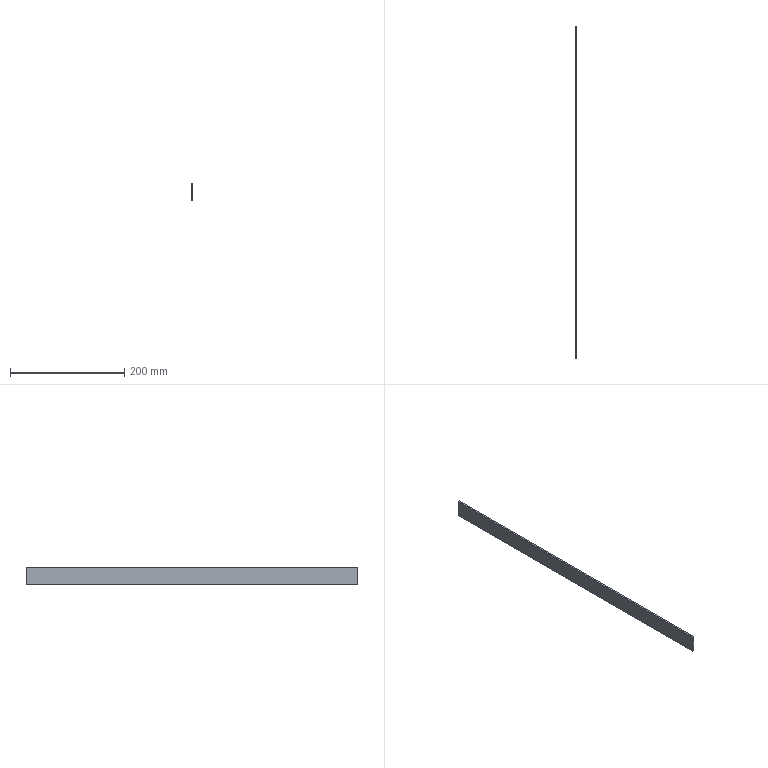Part | SolidWorks | 1 solid | 6 faces | box 3 x 582 x 30 mm | volume 52380 mm3 | plane 6
STEP:
#1=CARTESIAN_POINT('',(0.,291.,15.));
#2=VERTEX_POINT('',#1);
#3=CARTESIAN_POINT('',(0.,-291.,15.));
#4=VERTEX_POINT('',#3);
#5=CARTESIAN_POINT('',(0.,-291.,15.));
#6=DIRECTION('',(0.,-1.,0.));
#7=VECTOR('',#6,1000.);
#8=LINE('',#5,#7);
#9=EDGE_CURVE('',#2,#4,#8,.T.);
#10=ORIENTED_EDGE('',*,*,#9,.F.);
#11=CARTESIAN_POINT('',(-3.,291.,15.));
#12=VERTEX_POINT('',#11);
#13=CARTESIAN_POINT('',(-3.,291.,15.));
#14=DIRECTION('',(1.,0.,0.));
#15=VECTOR('',#14,1000.);
#16=LINE('',#13,#15);
#17=EDGE_CURVE('',#12,#2,#16,.T.);
#18=ORIENTED_EDGE('',*,*,#17,.F.);
#19=CARTESIAN_POINT('',(-3.,-291.,15.));
#20=VERTEX_POINT('',#19);
#21=CARTESIAN_POINT('',(-3.,-291.,15.));
#22=DIRECTION('',(0.,-1.,0.));
#23=VECTOR('',#22,1000.);
#24=LINE('',#21,#23);
#25=EDGE_CURVE('',#12,#20,#24,.T.);
#26=ORIENTED_EDGE('',*,*,#25,.T.);
#27=CARTESIAN_POINT('',(-3.,-291.,15.));
#28=DIRECTION('',(1.,0.,0.));
#29=VECTOR('',#28,1000.);
#30=LINE('',#27,#29);
#31=EDGE_CURVE('',#20,#4,#30,.T.);
#32=ORIENTED_EDGE('',*,*,#31,.T.);
#33=EDGE_LOOP('',(#10,#18,#26,#32));
#34=FACE_OUTER_BOUND('',#33,.T.);
#35=CARTESIAN_POINT('',(-3.,-291.,15.));
#36=DIRECTION('',(0.,0.,1.));
#37=DIRECTION('',(1.,0.,0.));
#38=AXIS2_PLACEMENT_3D('',#35,#36,#37);
#39=PLANE('',#38);
#40=ADVANCED_FACE('',(#34),#39,.T.);
#41=CARTESIAN_POINT('',(0.,291.,-15.));
#42=VERTEX_POINT('',#41);
#43=CARTESIAN_POINT('',(0.,291.,-15.));
#44=DIRECTION('',(0.,0.,1.));
#45=VECTOR('',#44,1000.);
#46=LINE('',#43,#45);
#47=EDGE_CURVE('',#42,#2,#46,.T.);
#48=ORIENTED_EDGE('',*,*,#47,.F.);
#49=CARTESIAN_POINT('',(-3.,291.,-15.));
#50=VERTEX_POINT('',#49);
#51=CARTESIAN_POINT('',(-3.,291.,-15.));
#52=DIRECTION('',(1.,0.,0.));
#53=VECTOR('',#52,1000.);
#54=LINE('',#51,#53);
#55=EDGE_CURVE('',#50,#42,#54,.T.);
#56=ORIENTED_EDGE('',*,*,#55,.F.);
#57=CARTESIAN_POINT('',(-3.,291.,-15.));
#58=DIRECTION('',(0.,0.,1.));
#59=VECTOR('',#58,1000.);
#60=LINE('',#57,#59);
#61=EDGE_CURVE('',#50,#12,#60,.T.);
#62=ORIENTED_EDGE('',*,*,#61,.T.);
#63=ORIENTED_EDGE('',*,*,#17,.T.);
#64=EDGE_LOOP('',(#48,#56,#62,#63));
#65=FACE_OUTER_BOUND('',#64,.T.);
#66=CARTESIAN_POINT('',(-3.,291.,-15.));
#67=DIRECTION('',(0.,1.,0.));
#68=DIRECTION('',(0.,0.,1.));
#69=AXIS2_PLACEMENT_3D('',#66,#67,#68);
#70=PLANE('',#69);
#71=ADVANCED_FACE('',(#65),#70,.T.);
#72=CARTESIAN_POINT('',(0.,-291.,-15.));
#73=VERTEX_POINT('',#72);
#74=CARTESIAN_POINT('',(0.,-291.,-15.));
#75=DIRECTION('',(0.,1.,0.));
#76=VECTOR('',#75,1000.);
#77=LINE('',#74,#76);
#78=EDGE_CURVE('',#73,#42,#77,.T.);
#79=ORIENTED_EDGE('',*,*,#78,.F.);
#80=CARTESIAN_POINT('',(-3.,-291.,-15.));
#81=VERTEX_POINT('',#80);
#82=CARTESIAN_POINT('',(-3.,-291.,-15.));
#83=DIRECTION('',(1.,0.,0.));
#84=VECTOR('',#83,1000.);
#85=LINE('',#82,#84);
#86=EDGE_CURVE('',#81,#73,#85,.T.);
#87=ORIENTED_EDGE('',*,*,#86,.F.);
#88=CARTESIAN_POINT('',(-3.,-291.,-15.));
#89=DIRECTION('',(0.,1.,0.));
#90=VECTOR('',#89,1000.);
#91=LINE('',#88,#90);
#92=EDGE_CURVE('',#81,#50,#91,.T.);
#93=ORIENTED_EDGE('',*,*,#92,.T.);
#94=ORIENTED_EDGE('',*,*,#55,.T.);
#95=EDGE_LOOP('',(#79,#87,#93,#94));
#96=FACE_OUTER_BOUND('',#95,.T.);
#97=CARTESIAN_POINT('',(-3.,-291.,-15.));
#98=DIRECTION('',(0.,0.,-1.));
#99=DIRECTION('',(-1.,0.,0.));
#100=AXIS2_PLACEMENT_3D('',#97,#98,#99);
#101=PLANE('',#100);
#102=ADVANCED_FACE('',(#96),#101,.T.);
#103=CARTESIAN_POINT('',(0.,-291.,-15.));
#104=DIRECTION('',(0.,0.,-1.));
#105=VECTOR('',#104,1000.);
#106=LINE('',#103,#105);
#107=EDGE_CURVE('',#4,#73,#106,.T.);
#108=ORIENTED_EDGE('',*,*,#107,.F.);
#109=ORIENTED_EDGE('',*,*,#31,.F.);
#110=CARTESIAN_POINT('',(-3.,-291.,-15.));
#111=DIRECTION('',(0.,0.,-1.));
#112=VECTOR('',#111,1000.);
#113=LINE('',#110,#112);
#114=EDGE_CURVE('',#20,#81,#113,.T.);
#115=ORIENTED_EDGE('',*,*,#114,.T.);
#116=ORIENTED_EDGE('',*,*,#86,.T.);
#117=EDGE_LOOP('',(#108,#109,#115,#116));
#118=FACE_OUTER_BOUND('',#117,.T.);
#119=CARTESIAN_POINT('',(-3.,-291.,-15.));
#120=DIRECTION('',(0.,-1.,0.));
#121=DIRECTION('',(0.,0.,-1.));
#122=AXIS2_PLACEMENT_3D('',#119,#120,#121);
#123=PLANE('',#122);
#124=ADVANCED_FACE('',(#118),#123,.T.);
#125=ORIENTED_EDGE('',*,*,#25,.F.);
#126=ORIENTED_EDGE('',*,*,#61,.F.);
#127=ORIENTED_EDGE('',*,*,#92,.F.);
#128=ORIENTED_EDGE('',*,*,#114,.F.);
#129=EDGE_LOOP('',(#125,#126,#127,#128));
#130=FACE_OUTER_BOUND('',#129,.T.);
#131=CARTESIAN_POINT('',(-3.,0.,0.));
#132=DIRECTION('',(1.,0.,0.));
#133=DIRECTION('',(0.,0.,-1.));
#134=AXIS2_PLACEMENT_3D('',#131,#132,#133);
#135=PLANE('',#134);
#136=ADVANCED_FACE('',(#130),#135,.F.);
#137=ORIENTED_EDGE('',*,*,#9,.T.);
#138=ORIENTED_EDGE('',*,*,#107,.T.);
#139=ORIENTED_EDGE('',*,*,#78,.T.);
#140=ORIENTED_EDGE('',*,*,#47,.T.);
#141=EDGE_LOOP('',(#137,#138,#139,#140));
#142=FACE_OUTER_BOUND('',#141,.T.);
#143=CARTESIAN_POINT('',(0.,0.,0.));
#144=DIRECTION('',(1.,0.,0.));
#145=DIRECTION('',(0.,0.,-1.));
#146=AXIS2_PLACEMENT_3D('',#143,#144,#145);
#147=PLANE('',#146);
#148=ADVANCED_FACE('',(#142),#147,.T.);
#149=CLOSED_SHELL('',(#40,#71,#102,#124,#136,#148));
#150=MANIFOLD_SOLID_BREP('',#149);
#151=CARTESIAN_POINT('',(0.,0.,0.));
#152=DIRECTION('',(0.,0.,1.));
#153=DIRECTION('',(1.,0.,0.));
#154=AXIS2_PLACEMENT_3D('',#151,#152,#153);
#155=(LENGTH_UNIT()NAMED_UNIT(*)SI_UNIT(.MILLI.,.METRE.));
#156=UNCERTAINTY_MEASURE_WITH_UNIT(LENGTH_MEASURE(0.00001),#155,'','');
#157=(NAMED_UNIT(*)PLANE_ANGLE_UNIT()SI_UNIT($,.RADIAN.));
#158=(NAMED_UNIT(*)SI_UNIT($,.STERADIAN.)SOLID_ANGLE_UNIT());
#159=(GEOMETRIC_REPRESENTATION_CONTEXT(3)GLOBAL_UNCERTAINTY_ASSIGNED_CONTEXT((#156))GLOBAL_UNIT_ASSIGNED_CONTEXT((#155,#157,#158))REPRESENTATION_CONTEXT('',''));
#160=ADVANCED_BREP_SHAPE_REPRESENTATION('',(#150,#154),#159);